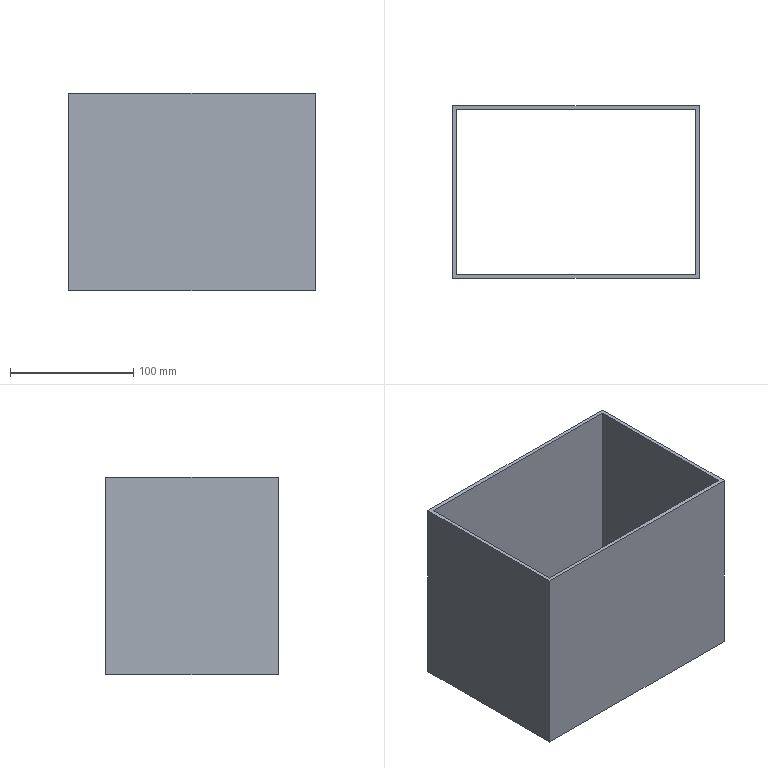Part | SolidWorks | features Extrusion 1 | 1 solid | 10 faces | box 200 x 140 x 160 mm | volume 320640 mm3 | plane 10
STEP:
#1=CARTESIAN_POINT('',(-100.,70.,80.));
#2=VERTEX_POINT('',#1);
#3=CARTESIAN_POINT('',(-100.,-70.,80.));
#4=VERTEX_POINT('',#3);
#5=CARTESIAN_POINT('',(-100.,70.,80.));
#6=DIRECTION('',(0.,-1.,0.));
#7=VECTOR('',#6,1000.);
#8=LINE('',#5,#7);
#9=EDGE_CURVE('',#2,#4,#8,.T.);
#10=ORIENTED_EDGE('',*,*,#9,.F.);
#11=CARTESIAN_POINT('',(-100.,70.,-80.));
#12=VERTEX_POINT('',#11);
#13=CARTESIAN_POINT('',(-100.,70.,-80.));
#14=DIRECTION('',(0.,0.,1.));
#15=VECTOR('',#14,1000.);
#16=LINE('',#13,#15);
#17=EDGE_CURVE('',#12,#2,#16,.T.);
#18=ORIENTED_EDGE('',*,*,#17,.F.);
#19=CARTESIAN_POINT('',(-100.,-70.,-80.));
#20=VERTEX_POINT('',#19);
#21=CARTESIAN_POINT('',(-100.,70.,-80.));
#22=DIRECTION('',(0.,-1.,0.));
#23=VECTOR('',#22,1000.);
#24=LINE('',#21,#23);
#25=EDGE_CURVE('',#12,#20,#24,.T.);
#26=ORIENTED_EDGE('',*,*,#25,.T.);
#27=CARTESIAN_POINT('',(-100.,-70.,-80.));
#28=DIRECTION('',(0.,0.,1.));
#29=VECTOR('',#28,1000.);
#30=LINE('',#27,#29);
#31=EDGE_CURVE('',#20,#4,#30,.T.);
#32=ORIENTED_EDGE('',*,*,#31,.T.);
#33=EDGE_LOOP('',(#10,#18,#26,#32));
#34=FACE_OUTER_BOUND('',#33,.T.);
#35=CARTESIAN_POINT('',(-100.,70.,-80.));
#36=DIRECTION('',(-1.,0.,0.));
#37=DIRECTION('',(0.,0.,1.));
#38=AXIS2_PLACEMENT_3D('',#35,#36,#37);
#39=PLANE('',#38);
#40=ADVANCED_FACE('',(#34),#39,.T.);
#41=CARTESIAN_POINT('',(100.,70.,80.));
#42=VERTEX_POINT('',#41);
#43=CARTESIAN_POINT('',(100.,70.,80.));
#44=DIRECTION('',(-1.,0.,0.));
#45=VECTOR('',#44,1000.);
#46=LINE('',#43,#45);
#47=EDGE_CURVE('',#42,#2,#46,.T.);
#48=ORIENTED_EDGE('',*,*,#47,.F.);
#49=CARTESIAN_POINT('',(100.,70.,-80.));
#50=VERTEX_POINT('',#49);
#51=CARTESIAN_POINT('',(100.,70.,-80.));
#52=DIRECTION('',(0.,0.,1.));
#53=VECTOR('',#52,1000.);
#54=LINE('',#51,#53);
#55=EDGE_CURVE('',#50,#42,#54,.T.);
#56=ORIENTED_EDGE('',*,*,#55,.F.);
#57=CARTESIAN_POINT('',(100.,70.,-80.));
#58=DIRECTION('',(-1.,0.,0.));
#59=VECTOR('',#58,1000.);
#60=LINE('',#57,#59);
#61=EDGE_CURVE('',#50,#12,#60,.T.);
#62=ORIENTED_EDGE('',*,*,#61,.T.);
#63=ORIENTED_EDGE('',*,*,#17,.T.);
#64=EDGE_LOOP('',(#48,#56,#62,#63));
#65=FACE_OUTER_BOUND('',#64,.T.);
#66=CARTESIAN_POINT('',(100.,70.,-80.));
#67=DIRECTION('',(0.,1.,0.));
#68=DIRECTION('',(0.,0.,1.));
#69=AXIS2_PLACEMENT_3D('',#66,#67,#68);
#70=PLANE('',#69);
#71=ADVANCED_FACE('',(#65),#70,.T.);
#72=CARTESIAN_POINT('',(100.,-70.,80.));
#73=VERTEX_POINT('',#72);
#74=CARTESIAN_POINT('',(100.,-70.,80.));
#75=DIRECTION('',(0.,1.,0.));
#76=VECTOR('',#75,1000.);
#77=LINE('',#74,#76);
#78=EDGE_CURVE('',#73,#42,#77,.T.);
#79=ORIENTED_EDGE('',*,*,#78,.F.);
#80=CARTESIAN_POINT('',(100.,-70.,-80.));
#81=VERTEX_POINT('',#80);
#82=CARTESIAN_POINT('',(100.,-70.,-80.));
#83=DIRECTION('',(0.,0.,1.));
#84=VECTOR('',#83,1000.);
#85=LINE('',#82,#84);
#86=EDGE_CURVE('',#81,#73,#85,.T.);
#87=ORIENTED_EDGE('',*,*,#86,.F.);
#88=CARTESIAN_POINT('',(100.,-70.,-80.));
#89=DIRECTION('',(0.,1.,0.));
#90=VECTOR('',#89,1000.);
#91=LINE('',#88,#90);
#92=EDGE_CURVE('',#81,#50,#91,.T.);
#93=ORIENTED_EDGE('',*,*,#92,.T.);
#94=ORIENTED_EDGE('',*,*,#55,.T.);
#95=EDGE_LOOP('',(#79,#87,#93,#94));
#96=FACE_OUTER_BOUND('',#95,.T.);
#97=CARTESIAN_POINT('',(100.,-70.,-80.));
#98=DIRECTION('',(1.,0.,0.));
#99=DIRECTION('',(0.,0.,-1.));
#100=AXIS2_PLACEMENT_3D('',#97,#98,#99);
#101=PLANE('',#100);
#102=ADVANCED_FACE('',(#96),#101,.T.);
#103=CARTESIAN_POINT('',(-100.,-70.,80.));
#104=DIRECTION('',(1.,0.,0.));
#105=VECTOR('',#104,1000.);
#106=LINE('',#103,#105);
#107=EDGE_CURVE('',#4,#73,#106,.T.);
#108=ORIENTED_EDGE('',*,*,#107,.F.);
#109=ORIENTED_EDGE('',*,*,#31,.F.);
#110=CARTESIAN_POINT('',(-100.,-70.,-80.));
#111=DIRECTION('',(1.,0.,0.));
#112=VECTOR('',#111,1000.);
#113=LINE('',#110,#112);
#114=EDGE_CURVE('',#20,#81,#113,.T.);
#115=ORIENTED_EDGE('',*,*,#114,.T.);
#116=ORIENTED_EDGE('',*,*,#86,.T.);
#117=EDGE_LOOP('',(#108,#109,#115,#116));
#118=FACE_OUTER_BOUND('',#117,.T.);
#119=CARTESIAN_POINT('',(-100.,-70.,-80.));
#120=DIRECTION('',(0.,-1.,0.));
#121=DIRECTION('',(0.,0.,-1.));
#122=AXIS2_PLACEMENT_3D('',#119,#120,#121);
#123=PLANE('',#122);
#124=ADVANCED_FACE('',(#118),#123,.T.);
#125=CARTESIAN_POINT('',(97.,67.,-80.));
#126=VERTEX_POINT('',#125);
#127=CARTESIAN_POINT('',(-97.,67.,-80.));
#128=VERTEX_POINT('',#127);
#129=CARTESIAN_POINT('',(97.,67.,-80.));
#130=DIRECTION('',(-1.,0.,0.));
#131=VECTOR('',#130,1000.);
#132=LINE('',#129,#131);
#133=EDGE_CURVE('',#126,#128,#132,.T.);
#134=ORIENTED_EDGE('',*,*,#133,.T.);
#135=CARTESIAN_POINT('',(-97.,-67.,-80.));
#136=VERTEX_POINT('',#135);
#137=CARTESIAN_POINT('',(-97.,67.,-80.));
#138=DIRECTION('',(0.,-1.,0.));
#139=VECTOR('',#138,1000.);
#140=LINE('',#137,#139);
#141=EDGE_CURVE('',#128,#136,#140,.T.);
#142=ORIENTED_EDGE('',*,*,#141,.T.);
#143=CARTESIAN_POINT('',(97.,-67.,-80.));
#144=VERTEX_POINT('',#143);
#145=CARTESIAN_POINT('',(-97.,-67.,-80.));
#146=DIRECTION('',(1.,0.,0.));
#147=VECTOR('',#146,1000.);
#148=LINE('',#145,#147);
#149=EDGE_CURVE('',#136,#144,#148,.T.);
#150=ORIENTED_EDGE('',*,*,#149,.T.);
#151=CARTESIAN_POINT('',(97.,-67.,-80.));
#152=DIRECTION('',(0.,1.,0.));
#153=VECTOR('',#152,1000.);
#154=LINE('',#151,#153);
#155=EDGE_CURVE('',#144,#126,#154,.T.);
#156=ORIENTED_EDGE('',*,*,#155,.T.);
#157=EDGE_LOOP('',(#134,#142,#150,#156));
#158=FACE_BOUND('',#157,.T.);
#159=ORIENTED_EDGE('',*,*,#25,.F.);
#160=ORIENTED_EDGE('',*,*,#61,.F.);
#161=ORIENTED_EDGE('',*,*,#92,.F.);
#162=ORIENTED_EDGE('',*,*,#114,.F.);
#163=EDGE_LOOP('',(#159,#160,#161,#162));
#164=FACE_OUTER_BOUND('',#163,.T.);
#165=CARTESIAN_POINT('',(0.,0.,-80.));
#166=DIRECTION('',(0.,0.,1.));
#167=DIRECTION('',(1.,0.,0.));
#168=AXIS2_PLACEMENT_3D('',#165,#166,#167);
#169=PLANE('',#168);
#170=ADVANCED_FACE('',(#158,#164),#169,.F.);
#171=CARTESIAN_POINT('',(-97.,67.,80.));
#172=VERTEX_POINT('',#171);
#173=CARTESIAN_POINT('',(-97.,-67.,80.));
#174=VERTEX_POINT('',#173);
#175=CARTESIAN_POINT('',(-97.,67.,80.));
#176=DIRECTION('',(0.,-1.,0.));
#177=VECTOR('',#176,1000.);
#178=LINE('',#175,#177);
#179=EDGE_CURVE('',#172,#174,#178,.T.);
#180=ORIENTED_EDGE('',*,*,#179,.F.);
#181=CARTESIAN_POINT('',(97.,67.,80.));
#182=VERTEX_POINT('',#181);
#183=CARTESIAN_POINT('',(97.,67.,80.));
#184=DIRECTION('',(-1.,0.,0.));
#185=VECTOR('',#184,1000.);
#186=LINE('',#183,#185);
#187=EDGE_CURVE('',#182,#172,#186,.T.);
#188=ORIENTED_EDGE('',*,*,#187,.F.);
#189=CARTESIAN_POINT('',(97.,-67.,80.));
#190=VERTEX_POINT('',#189);
#191=CARTESIAN_POINT('',(97.,-67.,80.));
#192=DIRECTION('',(0.,1.,0.));
#193=VECTOR('',#192,1000.);
#194=LINE('',#191,#193);
#195=EDGE_CURVE('',#190,#182,#194,.T.);
#196=ORIENTED_EDGE('',*,*,#195,.F.);
#197=CARTESIAN_POINT('',(-97.,-67.,80.));
#198=DIRECTION('',(1.,0.,0.));
#199=VECTOR('',#198,1000.);
#200=LINE('',#197,#199);
#201=EDGE_CURVE('',#174,#190,#200,.T.);
#202=ORIENTED_EDGE('',*,*,#201,.F.);
#203=EDGE_LOOP('',(#180,#188,#196,#202));
#204=FACE_BOUND('',#203,.T.);
#205=ORIENTED_EDGE('',*,*,#9,.T.);
#206=ORIENTED_EDGE('',*,*,#107,.T.);
#207=ORIENTED_EDGE('',*,*,#78,.T.);
#208=ORIENTED_EDGE('',*,*,#47,.T.);
#209=EDGE_LOOP('',(#205,#206,#207,#208));
#210=FACE_OUTER_BOUND('',#209,.T.);
#211=CARTESIAN_POINT('',(0.,0.,80.));
#212=DIRECTION('',(0.,0.,1.));
#213=DIRECTION('',(1.,0.,0.));
#214=AXIS2_PLACEMENT_3D('',#211,#212,#213);
#215=PLANE('',#214);
#216=ADVANCED_FACE('',(#204,#210),#215,.T.);
#217=ORIENTED_EDGE('',*,*,#179,.T.);
#218=CARTESIAN_POINT('',(-97.,-67.,-80.));
#219=DIRECTION('',(0.,0.,1.));
#220=VECTOR('',#219,1000.);
#221=LINE('',#218,#220);
#222=EDGE_CURVE('',#136,#174,#221,.T.);
#223=ORIENTED_EDGE('',*,*,#222,.F.);
#224=ORIENTED_EDGE('',*,*,#141,.F.);
#225=CARTESIAN_POINT('',(-97.,67.,-80.));
#226=DIRECTION('',(0.,0.,1.));
#227=VECTOR('',#226,1000.);
#228=LINE('',#225,#227);
#229=EDGE_CURVE('',#128,#172,#228,.T.);
#230=ORIENTED_EDGE('',*,*,#229,.T.);
#231=EDGE_LOOP('',(#217,#223,#224,#230));
#232=FACE_OUTER_BOUND('',#231,.T.);
#233=CARTESIAN_POINT('',(-97.,67.,-80.));
#234=DIRECTION('',(-1.,0.,0.));
#235=DIRECTION('',(0.,0.,1.));
#236=AXIS2_PLACEMENT_3D('',#233,#234,#235);
#237=PLANE('',#236);
#238=ADVANCED_FACE('',(#232),#237,.F.);
#239=ORIENTED_EDGE('',*,*,#187,.T.);
#240=ORIENTED_EDGE('',*,*,#229,.F.);
#241=ORIENTED_EDGE('',*,*,#133,.F.);
#242=CARTESIAN_POINT('',(97.,67.,-80.));
#243=DIRECTION('',(0.,0.,1.));
#244=VECTOR('',#243,1000.);
#245=LINE('',#242,#244);
#246=EDGE_CURVE('',#126,#182,#245,.T.);
#247=ORIENTED_EDGE('',*,*,#246,.T.);
#248=EDGE_LOOP('',(#239,#240,#241,#247));
#249=FACE_OUTER_BOUND('',#248,.T.);
#250=CARTESIAN_POINT('',(97.,67.,-80.));
#251=DIRECTION('',(0.,1.,0.));
#252=DIRECTION('',(0.,0.,1.));
#253=AXIS2_PLACEMENT_3D('',#250,#251,#252);
#254=PLANE('',#253);
#255=ADVANCED_FACE('',(#249),#254,.F.);
#256=ORIENTED_EDGE('',*,*,#195,.T.);
#257=ORIENTED_EDGE('',*,*,#246,.F.);
#258=ORIENTED_EDGE('',*,*,#155,.F.);
#259=CARTESIAN_POINT('',(97.,-67.,-80.));
#260=DIRECTION('',(0.,0.,1.));
#261=VECTOR('',#260,1000.);
#262=LINE('',#259,#261);
#263=EDGE_CURVE('',#144,#190,#262,.T.);
#264=ORIENTED_EDGE('',*,*,#263,.T.);
#265=EDGE_LOOP('',(#256,#257,#258,#264));
#266=FACE_OUTER_BOUND('',#265,.T.);
#267=CARTESIAN_POINT('',(97.,-67.,-80.));
#268=DIRECTION('',(1.,0.,0.));
#269=DIRECTION('',(0.,0.,-1.));
#270=AXIS2_PLACEMENT_3D('',#267,#268,#269);
#271=PLANE('',#270);
#272=ADVANCED_FACE('',(#266),#271,.F.);
#273=ORIENTED_EDGE('',*,*,#201,.T.);
#274=ORIENTED_EDGE('',*,*,#263,.F.);
#275=ORIENTED_EDGE('',*,*,#149,.F.);
#276=ORIENTED_EDGE('',*,*,#222,.T.);
#277=EDGE_LOOP('',(#273,#274,#275,#276));
#278=FACE_OUTER_BOUND('',#277,.T.);
#279=CARTESIAN_POINT('',(-97.,-67.,-80.));
#280=DIRECTION('',(0.,-1.,0.));
#281=DIRECTION('',(0.,0.,-1.));
#282=AXIS2_PLACEMENT_3D('',#279,#280,#281);
#283=PLANE('',#282);
#284=ADVANCED_FACE('',(#278),#283,.F.);
#285=CLOSED_SHELL('',(#40,#71,#102,#124,#170,#216,#238,#255,#272,#284));
#286=MANIFOLD_SOLID_BREP('',#285);
#287=CARTESIAN_POINT('',(0.,0.,0.));
#288=DIRECTION('',(0.,0.,1.));
#289=DIRECTION('',(1.,0.,0.));
#290=AXIS2_PLACEMENT_3D('',#287,#288,#289);
#291=(LENGTH_UNIT()NAMED_UNIT(*)SI_UNIT(.MILLI.,.METRE.));
#292=UNCERTAINTY_MEASURE_WITH_UNIT(LENGTH_MEASURE(0.00001),#291,'','');
#293=(NAMED_UNIT(*)PLANE_ANGLE_UNIT()SI_UNIT($,.RADIAN.));
#294=(NAMED_UNIT(*)SI_UNIT($,.STERADIAN.)SOLID_ANGLE_UNIT());
#295=(GEOMETRIC_REPRESENTATION_CONTEXT(3)GLOBAL_UNCERTAINTY_ASSIGNED_CONTEXT((#292))GLOBAL_UNIT_ASSIGNED_CONTEXT((#291,#293,#294))REPRESENTATION_CONTEXT('',''));
#296=ADVANCED_BREP_SHAPE_REPRESENTATION('',(#286,#290),#295);